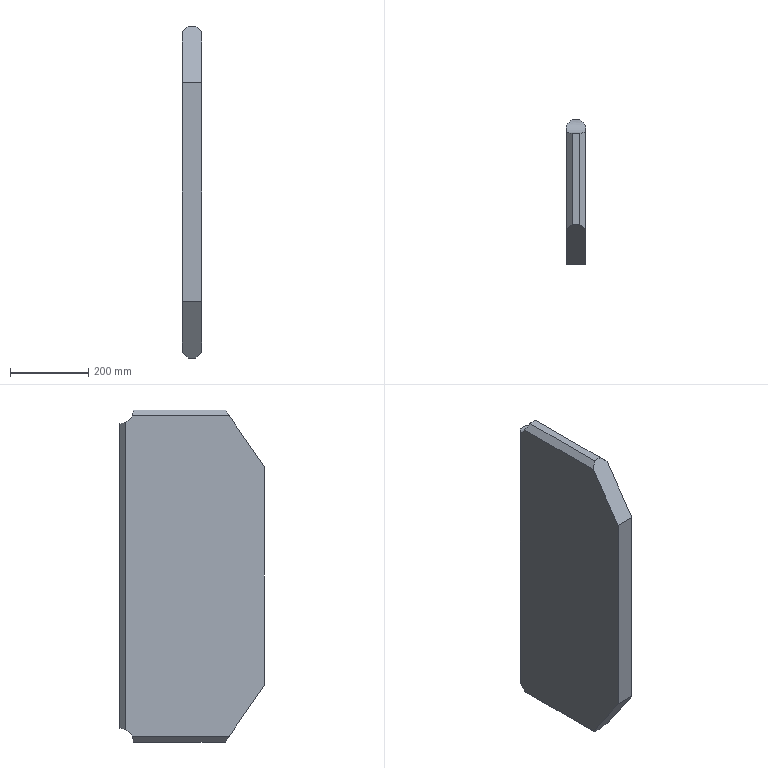Part | SolidWorks | features Chamfer 1, Extrusion 1 | 1 solid | 16 faces | box 50 x 370 x 850 mm | volume 14620496 mm3 | plane 14 | cylinder 2 | commonest cylinder face diameters 70 x2
STEP:
#1=CARTESIAN_POINT('',(-25.,338.377,-410.));
#2=VERTEX_POINT('',#1);
#3=CARTESIAN_POINT('',(-25.,355.,-393.377));
#4=VERTEX_POINT('',#3);
#5=CARTESIAN_POINT('',(-25.,370.,-425.));
#6=DIRECTION('',(-1.,0.,0.));
#7=DIRECTION('',(0.,0.,-1.));
#8=AXIS2_PLACEMENT_3D('',#5,#6,#7);
#9=CIRCLE('',#8,35.);
#10=EDGE_CURVE('',#2,#4,#9,.T.);
#11=ORIENTED_EDGE('',*,*,#10,.T.);
#12=CARTESIAN_POINT('',(-10.,370.,-390.));
#13=VERTEX_POINT('',#12);
#14=CARTESIAN_POINT('',(-25.,355.,-393.377));
#15=CARTESIAN_POINT('',(-20.293,359.707,-391.144));
#16=CARTESIAN_POINT('',(-15.21,364.79,-390.));
#17=CARTESIAN_POINT('',(-10.,370.,-390.));
#18=(BOUNDED_CURVE()B_SPLINE_CURVE(3,(#14,#15,#16,#17),.UNSPECIFIED.,.F.,.F.)B_SPLINE_CURVE_WITH_KNOTS((4,4),(1.128,1.571),.UNSPECIFIED.)CURVE()GEOMETRIC_REPRESENTATION_ITEM()RATIONAL_B_SPLINE_CURVE((1.,0.9837,0.9837,1.))REPRESENTATION_ITEM(''));
#19=EDGE_CURVE('',#4,#13,#18,.T.);
#20=ORIENTED_EDGE('',*,*,#19,.T.);
#21=CARTESIAN_POINT('',(10.,370.,-390.));
#22=VERTEX_POINT('',#21);
#23=CARTESIAN_POINT('',(25.,370.,-390.));
#24=DIRECTION('',(-1.,0.,0.));
#25=VECTOR('',#24,1000.);
#26=LINE('',#23,#25);
#27=EDGE_CURVE('',#22,#13,#26,.T.);
#28=ORIENTED_EDGE('',*,*,#27,.F.);
#29=CARTESIAN_POINT('',(25.,355.,-393.377));
#30=VERTEX_POINT('',#29);
#31=CARTESIAN_POINT('',(10.,370.,-390.));
#32=CARTESIAN_POINT('',(15.21,364.79,-390.));
#33=CARTESIAN_POINT('',(20.293,359.707,-391.144));
#34=CARTESIAN_POINT('',(25.,355.,-393.377));
#35=(BOUNDED_CURVE()B_SPLINE_CURVE(3,(#31,#32,#33,#34),.UNSPECIFIED.,.F.,.F.)B_SPLINE_CURVE_WITH_KNOTS((4,4),(1.571,2.014),.UNSPECIFIED.)CURVE()GEOMETRIC_REPRESENTATION_ITEM()RATIONAL_B_SPLINE_CURVE((1.,0.9837,0.9837,1.))REPRESENTATION_ITEM(''));
#36=EDGE_CURVE('',#22,#30,#35,.T.);
#37=ORIENTED_EDGE('',*,*,#36,.T.);
#38=CARTESIAN_POINT('',(25.,338.377,-410.));
#39=VERTEX_POINT('',#38);
#40=CARTESIAN_POINT('',(25.,370.,-425.));
#41=DIRECTION('',(-1.,0.,0.));
#42=DIRECTION('',(0.,0.,-1.));
#43=AXIS2_PLACEMENT_3D('',#40,#41,#42);
#44=CIRCLE('',#43,35.);
#45=EDGE_CURVE('',#39,#30,#44,.T.);
#46=ORIENTED_EDGE('',*,*,#45,.F.);
#47=CARTESIAN_POINT('',(10.,335.,-425.));
#48=VERTEX_POINT('',#47);
#49=CARTESIAN_POINT('',(25.,338.377,-410.));
#50=CARTESIAN_POINT('',(20.293,336.144,-414.707));
#51=CARTESIAN_POINT('',(15.21,335.,-419.79));
#52=CARTESIAN_POINT('',(10.,335.,-425.));
#53=(BOUNDED_CURVE()B_SPLINE_CURVE(3,(#49,#50,#51,#52),.UNSPECIFIED.,.F.,.F.)B_SPLINE_CURVE_WITH_KNOTS((4,4),(4.269,4.712),.UNSPECIFIED.)CURVE()GEOMETRIC_REPRESENTATION_ITEM()RATIONAL_B_SPLINE_CURVE((1.,0.9837,0.9837,1.))REPRESENTATION_ITEM(''));
#54=EDGE_CURVE('',#39,#48,#53,.T.);
#55=ORIENTED_EDGE('',*,*,#54,.T.);
#56=CARTESIAN_POINT('',(-10.,335.,-425.));
#57=VERTEX_POINT('',#56);
#58=CARTESIAN_POINT('',(25.,335.,-425.));
#59=DIRECTION('',(-1.,0.,0.));
#60=VECTOR('',#59,1000.);
#61=LINE('',#58,#60);
#62=EDGE_CURVE('',#48,#57,#61,.T.);
#63=ORIENTED_EDGE('',*,*,#62,.T.);
#64=CARTESIAN_POINT('',(-10.,335.,-425.));
#65=CARTESIAN_POINT('',(-15.21,335.,-419.79));
#66=CARTESIAN_POINT('',(-20.293,336.144,-414.707));
#67=CARTESIAN_POINT('',(-25.,338.377,-410.));
#68=(BOUNDED_CURVE()B_SPLINE_CURVE(3,(#64,#65,#66,#67),.UNSPECIFIED.,.F.,.T.)B_SPLINE_CURVE_WITH_KNOTS((4,4),(4.712,5.155),.UNSPECIFIED.)CURVE()GEOMETRIC_REPRESENTATION_ITEM()RATIONAL_B_SPLINE_CURVE((1.,0.9837,0.9837,1.))REPRESENTATION_ITEM(''));
#69=EDGE_CURVE('',#57,#2,#68,.T.);
#70=ORIENTED_EDGE('',*,*,#69,.T.);
#71=EDGE_LOOP('',(#11,#20,#28,#37,#46,#55,#63,#70));
#72=FACE_OUTER_BOUND('',#71,.T.);
#73=CARTESIAN_POINT('',(25.,370.,-425.));
#74=DIRECTION('',(-1.,0.,0.));
#75=DIRECTION('',(0.,0.,1.));
#76=AXIS2_PLACEMENT_3D('',#73,#74,#75);
#77=CYLINDRICAL_SURFACE('',#76,35.);
#78=ADVANCED_FACE('',(#72),#77,.F.);
#79=ORIENTED_EDGE('',*,*,#27,.T.);
#80=CARTESIAN_POINT('',(-10.,370.,390.));
#81=VERTEX_POINT('',#80);
#82=CARTESIAN_POINT('',(-10.,370.,390.));
#83=DIRECTION('',(0.,0.,1.));
#84=VECTOR('',#83,1000.);
#85=LINE('',#82,#84);
#86=EDGE_CURVE('',#13,#81,#85,.T.);
#87=ORIENTED_EDGE('',*,*,#86,.T.);
#88=CARTESIAN_POINT('',(10.,370.,390.));
#89=VERTEX_POINT('',#88);
#90=CARTESIAN_POINT('',(25.,370.,390.));
#91=DIRECTION('',(-1.,0.,0.));
#92=VECTOR('',#91,1000.);
#93=LINE('',#90,#92);
#94=EDGE_CURVE('',#89,#81,#93,.T.);
#95=ORIENTED_EDGE('',*,*,#94,.F.);
#96=CARTESIAN_POINT('',(10.,370.,-390.));
#97=DIRECTION('',(0.,0.,-1.));
#98=VECTOR('',#97,1000.);
#99=LINE('',#96,#98);
#100=EDGE_CURVE('',#89,#22,#99,.T.);
#101=ORIENTED_EDGE('',*,*,#100,.T.);
#102=EDGE_LOOP('',(#79,#87,#95,#101));
#103=FACE_OUTER_BOUND('',#102,.T.);
#104=CARTESIAN_POINT('',(25.,370.,390.));
#105=DIRECTION('',(0.,-1.,0.));
#106=DIRECTION('',(0.,0.,-1.));
#107=AXIS2_PLACEMENT_3D('',#104,#105,#106);
#108=PLANE('',#107);
#109=ADVANCED_FACE('',(#103),#108,.F.);
#110=CARTESIAN_POINT('',(-25.,355.,393.377));
#111=VERTEX_POINT('',#110);
#112=CARTESIAN_POINT('',(-25.,338.377,410.));
#113=VERTEX_POINT('',#112);
#114=CARTESIAN_POINT('',(-25.,370.,425.));
#115=DIRECTION('',(-1.,0.,0.));
#116=DIRECTION('',(0.,0.,1.));
#117=AXIS2_PLACEMENT_3D('',#114,#115,#116);
#118=CIRCLE('',#117,35.);
#119=EDGE_CURVE('',#111,#113,#118,.T.);
#120=ORIENTED_EDGE('',*,*,#119,.T.);
#121=CARTESIAN_POINT('',(-10.,335.,425.));
#122=VERTEX_POINT('',#121);
#123=CARTESIAN_POINT('',(-25.,338.377,410.));
#124=CARTESIAN_POINT('',(-20.293,336.144,414.707));
#125=CARTESIAN_POINT('',(-15.21,335.,419.79));
#126=CARTESIAN_POINT('',(-10.,335.,425.));
#127=(BOUNDED_CURVE()B_SPLINE_CURVE(3,(#123,#124,#125,#126),.UNSPECIFIED.,.F.,.F.)B_SPLINE_CURVE_WITH_KNOTS((4,4),(1.128,1.571),.UNSPECIFIED.)CURVE()GEOMETRIC_REPRESENTATION_ITEM()RATIONAL_B_SPLINE_CURVE((1.,0.9837,0.9837,1.))REPRESENTATION_ITEM(''));
#128=EDGE_CURVE('',#113,#122,#127,.T.);
#129=ORIENTED_EDGE('',*,*,#128,.T.);
#130=CARTESIAN_POINT('',(10.,335.,425.));
#131=VERTEX_POINT('',#130);
#132=CARTESIAN_POINT('',(25.,335.,425.));
#133=DIRECTION('',(-1.,0.,0.));
#134=VECTOR('',#133,1000.);
#135=LINE('',#132,#134);
#136=EDGE_CURVE('',#131,#122,#135,.T.);
#137=ORIENTED_EDGE('',*,*,#136,.F.);
#138=CARTESIAN_POINT('',(25.,338.377,410.));
#139=VERTEX_POINT('',#138);
#140=CARTESIAN_POINT('',(10.,335.,425.));
#141=CARTESIAN_POINT('',(15.21,335.,419.79));
#142=CARTESIAN_POINT('',(20.293,336.144,414.707));
#143=CARTESIAN_POINT('',(25.,338.377,410.));
#144=(BOUNDED_CURVE()B_SPLINE_CURVE(3,(#140,#141,#142,#143),.UNSPECIFIED.,.F.,.F.)B_SPLINE_CURVE_WITH_KNOTS((4,4),(1.571,2.014),.UNSPECIFIED.)CURVE()GEOMETRIC_REPRESENTATION_ITEM()RATIONAL_B_SPLINE_CURVE((1.,0.9837,0.9837,1.))REPRESENTATION_ITEM(''));
#145=EDGE_CURVE('',#131,#139,#144,.T.);
#146=ORIENTED_EDGE('',*,*,#145,.T.);
#147=CARTESIAN_POINT('',(25.,355.,393.377));
#148=VERTEX_POINT('',#147);
#149=CARTESIAN_POINT('',(25.,370.,425.));
#150=DIRECTION('',(-1.,0.,0.));
#151=DIRECTION('',(0.,0.,1.));
#152=AXIS2_PLACEMENT_3D('',#149,#150,#151);
#153=CIRCLE('',#152,35.);
#154=EDGE_CURVE('',#148,#139,#153,.T.);
#155=ORIENTED_EDGE('',*,*,#154,.F.);
#156=CARTESIAN_POINT('',(25.,355.,393.377));
#157=CARTESIAN_POINT('',(20.293,359.707,391.144));
#158=CARTESIAN_POINT('',(15.21,364.79,390.));
#159=CARTESIAN_POINT('',(10.,370.,390.));
#160=(BOUNDED_CURVE()B_SPLINE_CURVE(3,(#156,#157,#158,#159),.UNSPECIFIED.,.F.,.F.)B_SPLINE_CURVE_WITH_KNOTS((4,4),(4.269,4.712),.UNSPECIFIED.)CURVE()GEOMETRIC_REPRESENTATION_ITEM()RATIONAL_B_SPLINE_CURVE((1.,0.9837,0.9837,1.))REPRESENTATION_ITEM(''));
#161=EDGE_CURVE('',#148,#89,#160,.T.);
#162=ORIENTED_EDGE('',*,*,#161,.T.);
#163=ORIENTED_EDGE('',*,*,#94,.T.);
#164=CARTESIAN_POINT('',(-10.,370.,390.));
#165=CARTESIAN_POINT('',(-15.21,364.79,390.));
#166=CARTESIAN_POINT('',(-20.293,359.707,391.144));
#167=CARTESIAN_POINT('',(-25.,355.,393.377));
#168=(BOUNDED_CURVE()B_SPLINE_CURVE(3,(#164,#165,#166,#167),.UNSPECIFIED.,.F.,.F.)B_SPLINE_CURVE_WITH_KNOTS((4,4),(4.712,5.155),.UNSPECIFIED.)CURVE()GEOMETRIC_REPRESENTATION_ITEM()RATIONAL_B_SPLINE_CURVE((1.,0.9837,0.9837,1.))REPRESENTATION_ITEM(''));
#169=EDGE_CURVE('',#81,#111,#168,.T.);
#170=ORIENTED_EDGE('',*,*,#169,.T.);
#171=EDGE_LOOP('',(#120,#129,#137,#146,#155,#162,#163,#170));
#172=FACE_OUTER_BOUND('',#171,.T.);
#173=CARTESIAN_POINT('',(25.,370.,425.));
#174=DIRECTION('',(-1.,0.,0.));
#175=DIRECTION('',(0.,0.,1.));
#176=AXIS2_PLACEMENT_3D('',#173,#174,#175);
#177=CYLINDRICAL_SURFACE('',#176,35.);
#178=ADVANCED_FACE('',(#172),#177,.F.);
#179=ORIENTED_EDGE('',*,*,#136,.T.);
#180=CARTESIAN_POINT('',(-10.,100.,425.));
#181=VERTEX_POINT('',#180);
#182=CARTESIAN_POINT('',(-10.,335.,425.));
#183=DIRECTION('',(0.,-1.,0.));
#184=VECTOR('',#183,1000.);
#185=LINE('',#182,#184);
#186=EDGE_CURVE('',#122,#181,#185,.T.);
#187=ORIENTED_EDGE('',*,*,#186,.T.);
#188=CARTESIAN_POINT('',(10.,100.,425.));
#189=VERTEX_POINT('',#188);
#190=CARTESIAN_POINT('',(25.,100.,425.));
#191=DIRECTION('',(-1.,0.,0.));
#192=VECTOR('',#191,1000.);
#193=LINE('',#190,#192);
#194=EDGE_CURVE('',#189,#181,#193,.T.);
#195=ORIENTED_EDGE('',*,*,#194,.F.);
#196=CARTESIAN_POINT('',(10.,335.,425.));
#197=DIRECTION('',(0.,1.,0.));
#198=VECTOR('',#197,1000.);
#199=LINE('',#196,#198);
#200=EDGE_CURVE('',#189,#131,#199,.T.);
#201=ORIENTED_EDGE('',*,*,#200,.T.);
#202=EDGE_LOOP('',(#179,#187,#195,#201));
#203=FACE_OUTER_BOUND('',#202,.T.);
#204=CARTESIAN_POINT('',(25.,335.,425.));
#205=DIRECTION('',(0.,0.,-1.));
#206=DIRECTION('',(0.,1.,0.));
#207=AXIS2_PLACEMENT_3D('',#204,#205,#206);
#208=PLANE('',#207);
#209=ADVANCED_FACE('',(#203),#208,.F.);
#210=ORIENTED_EDGE('',*,*,#194,.T.);
#211=CARTESIAN_POINT('',(-25.,89.655,410.));
#212=VERTEX_POINT('',#211);
#213=CARTESIAN_POINT('',(55.466,145.149,490.466));
#214=DIRECTION('',(-0.6356,-0.4383,-0.6356));
#215=VECTOR('',#214,1000.);
#216=LINE('',#213,#215);
#217=EDGE_CURVE('',#181,#212,#216,.T.);
#218=ORIENTED_EDGE('',*,*,#217,.T.);
#219=CARTESIAN_POINT('',(-25.,0.,280.));
#220=VERTEX_POINT('',#219);
#221=CARTESIAN_POINT('',(-25.,100.,425.));
#222=DIRECTION('',(0.,-0.5677,-0.8232));
#223=VECTOR('',#222,1000.);
#224=LINE('',#221,#223);
#225=EDGE_CURVE('',#212,#220,#224,.T.);
#226=ORIENTED_EDGE('',*,*,#225,.T.);
#227=CARTESIAN_POINT('',(25.,0.,280.));
#228=VERTEX_POINT('',#227);
#229=CARTESIAN_POINT('',(25.,0.,280.));
#230=DIRECTION('',(-1.,0.,0.));
#231=VECTOR('',#230,1000.);
#232=LINE('',#229,#231);
#233=EDGE_CURVE('',#228,#220,#232,.T.);
#234=ORIENTED_EDGE('',*,*,#233,.F.);
#235=CARTESIAN_POINT('',(25.,89.655,410.));
#236=VERTEX_POINT('',#235);
#237=CARTESIAN_POINT('',(25.,100.,425.));
#238=DIRECTION('',(0.,-0.5677,-0.8232));
#239=VECTOR('',#238,1000.);
#240=LINE('',#237,#239);
#241=EDGE_CURVE('',#236,#228,#240,.T.);
#242=ORIENTED_EDGE('',*,*,#241,.F.);
#243=CARTESIAN_POINT('',(-53.098,143.516,488.098));
#244=DIRECTION('',(-0.6356,0.4383,0.6356));
#245=VECTOR('',#244,1000.);
#246=LINE('',#243,#245);
#247=EDGE_CURVE('',#236,#189,#246,.T.);
#248=ORIENTED_EDGE('',*,*,#247,.T.);
#249=EDGE_LOOP('',(#210,#218,#226,#234,#242,#248));
#250=FACE_OUTER_BOUND('',#249,.T.);
#251=CARTESIAN_POINT('',(25.,100.,425.));
#252=DIRECTION('',(0.,0.8232,-0.5677));
#253=DIRECTION('',(0.,0.5677,0.8232));
#254=AXIS2_PLACEMENT_3D('',#251,#252,#253);
#255=PLANE('',#254);
#256=ADVANCED_FACE('',(#250),#255,.F.);
#257=CARTESIAN_POINT('',(-25.,0.,-280.));
#258=VERTEX_POINT('',#257);
#259=CARTESIAN_POINT('',(-25.,0.,-280.));
#260=DIRECTION('',(0.,0.,-1.));
#261=VECTOR('',#260,1000.);
#262=LINE('',#259,#261);
#263=EDGE_CURVE('',#220,#258,#262,.T.);
#264=ORIENTED_EDGE('',*,*,#263,.T.);
#265=CARTESIAN_POINT('',(25.,0.,-280.));
#266=VERTEX_POINT('',#265);
#267=CARTESIAN_POINT('',(25.,0.,-280.));
#268=DIRECTION('',(-1.,0.,0.));
#269=VECTOR('',#268,1000.);
#270=LINE('',#267,#269);
#271=EDGE_CURVE('',#266,#258,#270,.T.);
#272=ORIENTED_EDGE('',*,*,#271,.F.);
#273=CARTESIAN_POINT('',(25.,0.,-280.));
#274=DIRECTION('',(0.,0.,-1.));
#275=VECTOR('',#274,1000.);
#276=LINE('',#273,#275);
#277=EDGE_CURVE('',#228,#266,#276,.T.);
#278=ORIENTED_EDGE('',*,*,#277,.F.);
#279=ORIENTED_EDGE('',*,*,#233,.T.);
#280=EDGE_LOOP('',(#264,#272,#278,#279));
#281=FACE_OUTER_BOUND('',#280,.T.);
#282=CARTESIAN_POINT('',(25.,0.,-280.));
#283=DIRECTION('',(0.,1.,0.));
#284=DIRECTION('',(0.,0.,1.));
#285=AXIS2_PLACEMENT_3D('',#282,#283,#284);
#286=PLANE('',#285);
#287=ADVANCED_FACE('',(#281),#286,.F.);
#288=CARTESIAN_POINT('',(-25.,89.655,-410.));
#289=VERTEX_POINT('',#288);
#290=CARTESIAN_POINT('',(-25.,100.,-425.));
#291=DIRECTION('',(0.,0.5677,-0.8232));
#292=VECTOR('',#291,1000.);
#293=LINE('',#290,#292);
#294=EDGE_CURVE('',#258,#289,#293,.T.);
#295=ORIENTED_EDGE('',*,*,#294,.T.);
#296=CARTESIAN_POINT('',(-10.,100.,-425.));
#297=VERTEX_POINT('',#296);
#298=CARTESIAN_POINT('',(55.466,145.149,-490.466));
#299=DIRECTION('',(0.6356,0.4383,-0.6356));
#300=VECTOR('',#299,1000.);
#301=LINE('',#298,#300);
#302=EDGE_CURVE('',#289,#297,#301,.T.);
#303=ORIENTED_EDGE('',*,*,#302,.T.);
#304=CARTESIAN_POINT('',(10.,100.,-425.));
#305=VERTEX_POINT('',#304);
#306=CARTESIAN_POINT('',(25.,100.,-425.));
#307=DIRECTION('',(-1.,0.,0.));
#308=VECTOR('',#307,1000.);
#309=LINE('',#306,#308);
#310=EDGE_CURVE('',#305,#297,#309,.T.);
#311=ORIENTED_EDGE('',*,*,#310,.F.);
#312=CARTESIAN_POINT('',(25.,89.655,-410.));
#313=VERTEX_POINT('',#312);
#314=CARTESIAN_POINT('',(-53.098,143.516,-488.098));
#315=DIRECTION('',(0.6356,-0.4383,0.6356));
#316=VECTOR('',#315,1000.);
#317=LINE('',#314,#316);
#318=EDGE_CURVE('',#305,#313,#317,.T.);
#319=ORIENTED_EDGE('',*,*,#318,.T.);
#320=CARTESIAN_POINT('',(25.,100.,-425.));
#321=DIRECTION('',(0.,0.5677,-0.8232));
#322=VECTOR('',#321,1000.);
#323=LINE('',#320,#322);
#324=EDGE_CURVE('',#266,#313,#323,.T.);
#325=ORIENTED_EDGE('',*,*,#324,.F.);
#326=ORIENTED_EDGE('',*,*,#271,.T.);
#327=EDGE_LOOP('',(#295,#303,#311,#319,#325,#326));
#328=FACE_OUTER_BOUND('',#327,.T.);
#329=CARTESIAN_POINT('',(25.,100.,-425.));
#330=DIRECTION('',(0.,0.8232,0.5677));
#331=DIRECTION('',(0.,-0.5677,0.8232));
#332=AXIS2_PLACEMENT_3D('',#329,#330,#331);
#333=PLANE('',#332);
#334=ADVANCED_FACE('',(#328),#333,.F.);
#335=ORIENTED_EDGE('',*,*,#310,.T.);
#336=CARTESIAN_POINT('',(-10.,335.,-425.));
#337=DIRECTION('',(0.,1.,0.));
#338=VECTOR('',#337,1000.);
#339=LINE('',#336,#338);
#340=EDGE_CURVE('',#297,#57,#339,.T.);
#341=ORIENTED_EDGE('',*,*,#340,.T.);
#342=ORIENTED_EDGE('',*,*,#62,.F.);
#343=CARTESIAN_POINT('',(10.,100.,-425.));
#344=DIRECTION('',(0.,-1.,0.));
#345=VECTOR('',#344,1000.);
#346=LINE('',#343,#345);
#347=EDGE_CURVE('',#48,#305,#346,.T.);
#348=ORIENTED_EDGE('',*,*,#347,.T.);
#349=EDGE_LOOP('',(#335,#341,#342,#348));
#350=FACE_OUTER_BOUND('',#349,.T.);
#351=CARTESIAN_POINT('',(25.,335.,-425.));
#352=DIRECTION('',(0.,0.,1.));
#353=DIRECTION('',(0.,-1.,0.));
#354=AXIS2_PLACEMENT_3D('',#351,#352,#353);
#355=PLANE('',#354);
#356=ADVANCED_FACE('',(#350),#355,.F.);
#357=ORIENTED_EDGE('',*,*,#324,.T.);
#358=CARTESIAN_POINT('',(25.,335.,-410.));
#359=DIRECTION('',(0.,1.,0.));
#360=VECTOR('',#359,1000.);
#361=LINE('',#358,#360);
#362=EDGE_CURVE('',#313,#39,#361,.T.);
#363=ORIENTED_EDGE('',*,*,#362,.T.);
#364=ORIENTED_EDGE('',*,*,#45,.T.);
#365=CARTESIAN_POINT('',(25.,355.,390.));
#366=DIRECTION('',(0.,0.,1.));
#367=VECTOR('',#366,1000.);
#368=LINE('',#365,#367);
#369=EDGE_CURVE('',#30,#148,#368,.T.);
#370=ORIENTED_EDGE('',*,*,#369,.T.);
#371=ORIENTED_EDGE('',*,*,#154,.T.);
#372=CARTESIAN_POINT('',(25.,100.,410.));
#373=DIRECTION('',(0.,-1.,0.));
#374=VECTOR('',#373,1000.);
#375=LINE('',#372,#374);
#376=EDGE_CURVE('',#139,#236,#375,.T.);
#377=ORIENTED_EDGE('',*,*,#376,.T.);
#378=ORIENTED_EDGE('',*,*,#241,.T.);
#379=ORIENTED_EDGE('',*,*,#277,.T.);
#380=EDGE_LOOP('',(#357,#363,#364,#370,#371,#377,#378,#379));
#381=FACE_OUTER_BOUND('',#380,.T.);
#382=CARTESIAN_POINT('',(25.,370.,-425.));
#383=DIRECTION('',(1.,0.,0.));
#384=DIRECTION('',(0.,0.,-1.));
#385=AXIS2_PLACEMENT_3D('',#382,#383,#384);
#386=PLANE('',#385);
#387=ADVANCED_FACE('',(#381),#386,.T.);
#388=ORIENTED_EDGE('',*,*,#225,.F.);
#389=CARTESIAN_POINT('',(-25.,370.,410.));
#390=DIRECTION('',(0.,1.,0.));
#391=VECTOR('',#390,1000.);
#392=LINE('',#389,#391);
#393=EDGE_CURVE('',#212,#113,#392,.T.);
#394=ORIENTED_EDGE('',*,*,#393,.T.);
#395=ORIENTED_EDGE('',*,*,#119,.F.);
#396=CARTESIAN_POINT('',(-25.,355.,-425.));
#397=DIRECTION('',(0.,0.,-1.));
#398=VECTOR('',#397,1000.);
#399=LINE('',#396,#398);
#400=EDGE_CURVE('',#111,#4,#399,.T.);
#401=ORIENTED_EDGE('',*,*,#400,.T.);
#402=ORIENTED_EDGE('',*,*,#10,.F.);
#403=CARTESIAN_POINT('',(-25.,370.,-410.));
#404=DIRECTION('',(0.,-1.,0.));
#405=VECTOR('',#404,1000.);
#406=LINE('',#403,#405);
#407=EDGE_CURVE('',#2,#289,#406,.T.);
#408=ORIENTED_EDGE('',*,*,#407,.T.);
#409=ORIENTED_EDGE('',*,*,#294,.F.);
#410=ORIENTED_EDGE('',*,*,#263,.F.);
#411=EDGE_LOOP('',(#388,#394,#395,#401,#402,#408,#409,#410));
#412=FACE_OUTER_BOUND('',#411,.T.);
#413=CARTESIAN_POINT('',(-25.,370.,-425.));
#414=DIRECTION('',(1.,0.,0.));
#415=DIRECTION('',(0.,0.,-1.));
#416=AXIS2_PLACEMENT_3D('',#413,#414,#415);
#417=PLANE('',#416);
#418=ADVANCED_FACE('',(#412),#417,.F.);
#419=ORIENTED_EDGE('',*,*,#128,.F.);
#420=ORIENTED_EDGE('',*,*,#393,.F.);
#421=ORIENTED_EDGE('',*,*,#217,.F.);
#422=ORIENTED_EDGE('',*,*,#186,.F.);
#423=EDGE_LOOP('',(#419,#420,#421,#422));
#424=FACE_OUTER_BOUND('',#423,.T.);
#425=CARTESIAN_POINT('',(-10.,335.,425.));
#426=DIRECTION('',(0.7071,0.,-0.7071));
#427=DIRECTION('',(0.,-1.,0.));
#428=AXIS2_PLACEMENT_3D('',#425,#426,#427);
#429=PLANE('',#428);
#430=ADVANCED_FACE('',(#424),#429,.F.);
#431=ORIENTED_EDGE('',*,*,#19,.F.);
#432=ORIENTED_EDGE('',*,*,#400,.F.);
#433=ORIENTED_EDGE('',*,*,#169,.F.);
#434=ORIENTED_EDGE('',*,*,#86,.F.);
#435=EDGE_LOOP('',(#431,#432,#433,#434));
#436=FACE_OUTER_BOUND('',#435,.T.);
#437=CARTESIAN_POINT('',(-10.,370.,390.));
#438=DIRECTION('',(0.7071,-0.7071,0.));
#439=DIRECTION('',(0.,0.,1.));
#440=AXIS2_PLACEMENT_3D('',#437,#438,#439);
#441=PLANE('',#440);
#442=ADVANCED_FACE('',(#436),#441,.F.);
#443=ORIENTED_EDGE('',*,*,#302,.F.);
#444=ORIENTED_EDGE('',*,*,#407,.F.);
#445=ORIENTED_EDGE('',*,*,#69,.F.);
#446=ORIENTED_EDGE('',*,*,#340,.F.);
#447=EDGE_LOOP('',(#443,#444,#445,#446));
#448=FACE_OUTER_BOUND('',#447,.T.);
#449=CARTESIAN_POINT('',(-10.,335.,-425.));
#450=DIRECTION('',(0.7071,0.,0.7071));
#451=DIRECTION('',(0.,1.,0.));
#452=AXIS2_PLACEMENT_3D('',#449,#450,#451);
#453=PLANE('',#452);
#454=ADVANCED_FACE('',(#448),#453,.F.);
#455=ORIENTED_EDGE('',*,*,#318,.F.);
#456=ORIENTED_EDGE('',*,*,#347,.F.);
#457=ORIENTED_EDGE('',*,*,#54,.F.);
#458=ORIENTED_EDGE('',*,*,#362,.F.);
#459=EDGE_LOOP('',(#455,#456,#457,#458));
#460=FACE_OUTER_BOUND('',#459,.T.);
#461=CARTESIAN_POINT('',(25.,370.,-410.));
#462=DIRECTION('',(0.7071,0.,-0.7071));
#463=DIRECTION('',(0.,-1.,0.));
#464=AXIS2_PLACEMENT_3D('',#461,#462,#463);
#465=PLANE('',#464);
#466=ADVANCED_FACE('',(#460),#465,.T.);
#467=ORIENTED_EDGE('',*,*,#36,.F.);
#468=ORIENTED_EDGE('',*,*,#100,.F.);
#469=ORIENTED_EDGE('',*,*,#161,.F.);
#470=ORIENTED_EDGE('',*,*,#369,.F.);
#471=EDGE_LOOP('',(#467,#468,#469,#470));
#472=FACE_OUTER_BOUND('',#471,.T.);
#473=CARTESIAN_POINT('',(25.,355.,-425.));
#474=DIRECTION('',(0.7071,0.7071,0.));
#475=DIRECTION('',(0.,0.,-1.));
#476=AXIS2_PLACEMENT_3D('',#473,#474,#475);
#477=PLANE('',#476);
#478=ADVANCED_FACE('',(#472),#477,.T.);
#479=ORIENTED_EDGE('',*,*,#145,.F.);
#480=ORIENTED_EDGE('',*,*,#200,.F.);
#481=ORIENTED_EDGE('',*,*,#247,.F.);
#482=ORIENTED_EDGE('',*,*,#376,.F.);
#483=EDGE_LOOP('',(#479,#480,#481,#482));
#484=FACE_OUTER_BOUND('',#483,.T.);
#485=CARTESIAN_POINT('',(25.,370.,410.));
#486=DIRECTION('',(0.7071,0.,0.7071));
#487=DIRECTION('',(0.,1.,0.));
#488=AXIS2_PLACEMENT_3D('',#485,#486,#487);
#489=PLANE('',#488);
#490=ADVANCED_FACE('',(#484),#489,.T.);
#491=CLOSED_SHELL('',(#78,#109,#178,#209,#256,#287,#334,#356,#387,#418,#430,#442,#454,#466,#478,#490));
#492=MANIFOLD_SOLID_BREP('',#491);
#493=CARTESIAN_POINT('',(0.,0.,0.));
#494=DIRECTION('',(0.,0.,1.));
#495=DIRECTION('',(1.,0.,0.));
#496=AXIS2_PLACEMENT_3D('',#493,#494,#495);
#497=(LENGTH_UNIT()NAMED_UNIT(*)SI_UNIT(.MILLI.,.METRE.));
#498=UNCERTAINTY_MEASURE_WITH_UNIT(LENGTH_MEASURE(0.00001),#497,'','');
#499=(NAMED_UNIT(*)PLANE_ANGLE_UNIT()SI_UNIT($,.RADIAN.));
#500=(NAMED_UNIT(*)SI_UNIT($,.STERADIAN.)SOLID_ANGLE_UNIT());
#501=(GEOMETRIC_REPRESENTATION_CONTEXT(3)GLOBAL_UNCERTAINTY_ASSIGNED_CONTEXT((#498))GLOBAL_UNIT_ASSIGNED_CONTEXT((#497,#499,#500))REPRESENTATION_CONTEXT('',''));
#502=ADVANCED_BREP_SHAPE_REPRESENTATION('',(#492,#496),#501);